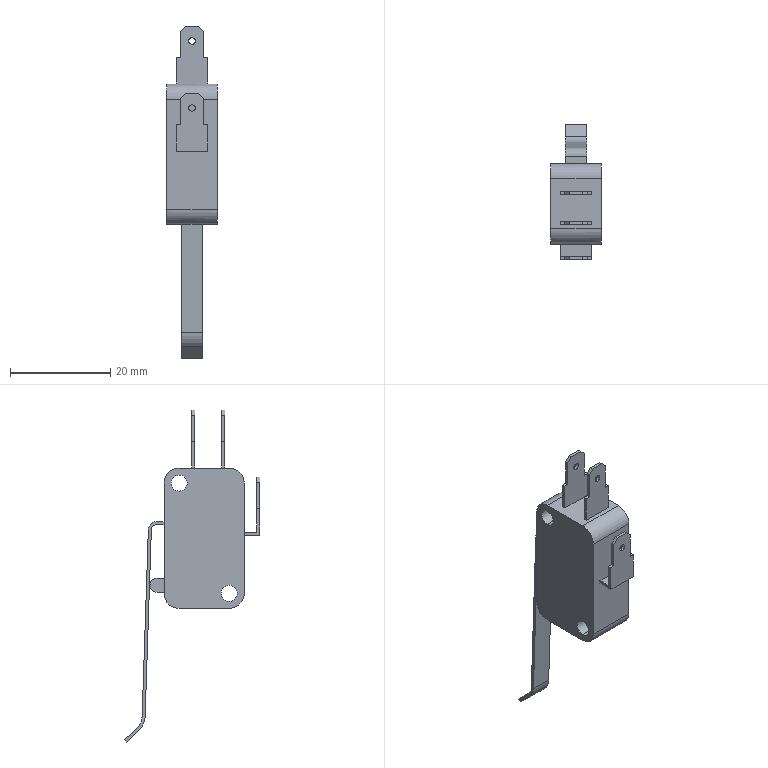Part | STEP file | 102000010521 | 1 solid | 74 faces | box 10 x 27.034 x 66.257 mm | volume 4509 mm3 | plane 54 | cylinder 20 | commonest cylinder face diameters 1.3 x6 3.2 x5 6 x4 2.8 x2 2 x1 6.8 x1